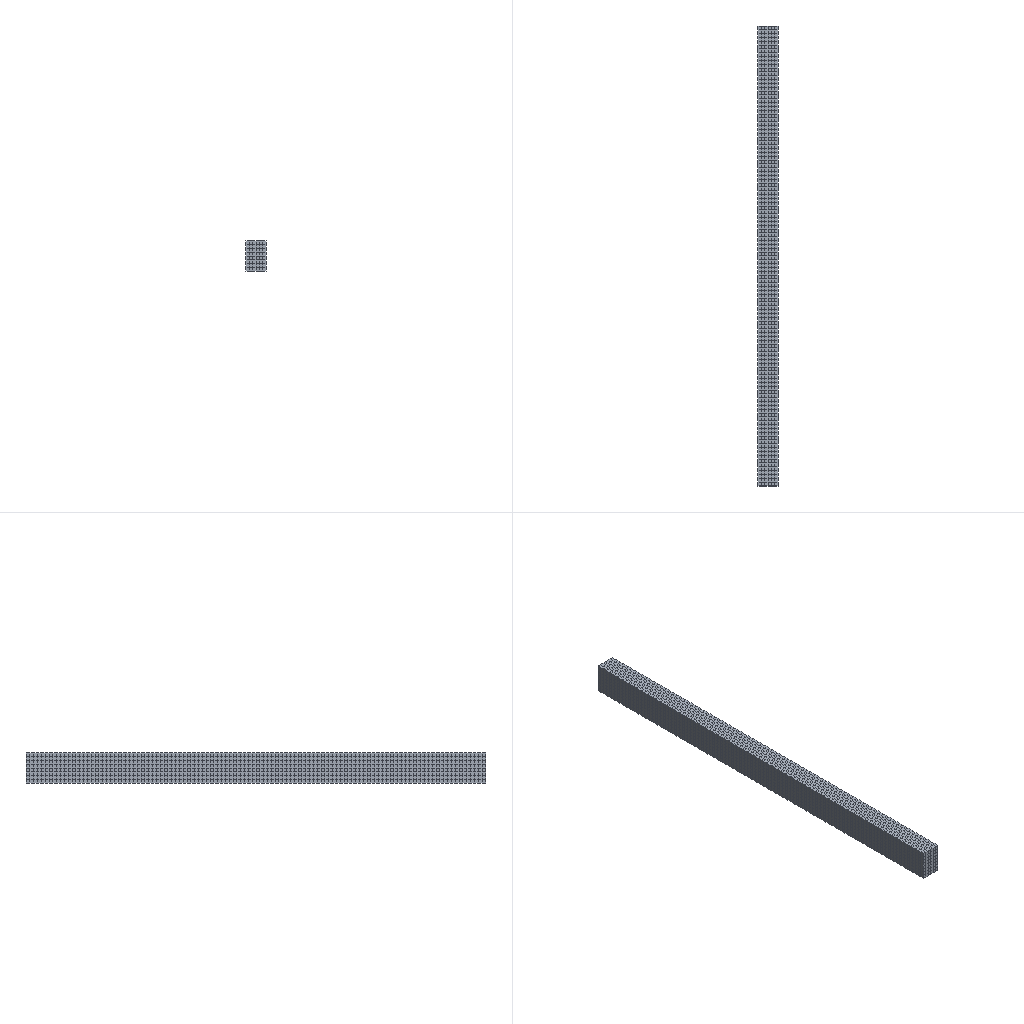Simulation study | ansys workbench
Ansys APDL input file, long lists of numbers shortened:
/batch
/config,noeldb,1     ! force off writing results to database
*get,_wallstrt,active,,time,wall
! ANSYS input file written by Workbench version 2022 R1
! File used for geometry attach: F:\ansys（分析文件汇总)\简支梁有限元分析\零件3.STEP
/title,111--____ (C5)
! ****** Begin Custom Load Command Snippet ******
/COM, ACT Extensions:
/COM,     LSDYNA, 2021.1
/COM,
! ****** End   Custom Load Command Snippet ******
*DIM,_wb_ProjectScratch_dir,string,248
_wb_ProjectScratch_dir(1) = 'F:\ansys（分析文件汇总)\简支梁有限元分析\_ProjectScratch\ScrC7EA\'
*DIM,_wb_SolverFiles_dir,string,248
_wb_SolverFiles_dir(1) = 'F:\ansys（分析文件汇总)\简支梁有限元分析\111_files\dp0\SYS-1\MECH\'
*DIM,_wb_userfiles_dir,string,248
_wb_userfiles_dir(1) = 'F:\ansys（分析文件汇总)\简支梁有限元分析\111_files\user_files\'
/com,--- Data in consistent NMM units. See Solving Units in the help system for more information.
/units,MPA
/nopr
/wb,file,start              !  signify a WB generated input file
/prep7
! Turn off shape checking because checks already performed inside WB mesher.
! See help system for more information.
SHPP,OFF,,NOWARN
/nolist
etcon,set             ! allow ANSYS to choose best KEYOP's for 180x elements, resets any applicable keyopt to MAPDL defaults
/com,*********** Nodes for the whole assembly ***********
nblock,3,,127902
(1i9,3e20.9e3)
        1    -5.133333333E+01     1.215000000E+03     8.485714286E+01
! (116274 more lines like these left out)
-1
/wb,elem,start            !  set before creation of elements
/com,*********** Elements for Body 1 "__3-FreeParts|__1[2]" ***********
et,1,186
keyo,1,2,1          ! set full integration on SOLID186
eblock,19,solid,,10080
(19i9)
        1        1        1        1        0        0        0        0       20        0    15121    69851    80547    80568    81290    79093    80560    80569    82000
! (20159 more lines like these left out)
-1
/com,*********** Elements for Body 2 "__3-FreeParts|__1[1]" ***********
et,2,186
keyo,2,2,1          ! set full integration on SOLID186
eblock,19,solid,,5040
(19i9)
        2        2        2        2        0        0        0        0       20        0        1        1     5405     5441     5449     4563     5418     5440     5799
! (10079 more lines like these left out)
-1
/com,*********** Elements for Body 3 "__3-FreeParts|__1[3]" ***********
et,3,186
keyo,3,2,1          ! set full integration on SOLID186
eblock,19,solid,,10080
(19i9)
        3        3        3        3        0        0        0        0       20        0     5041    23426    35471    34596    34515    32668    35563    34595    34594
! (20159 more lines like these left out)
-1
/wb,elem,end               !  done creating elements
/com,*********** Send User Defined Coordinate System(s) ***********
csys,0
toffst,273.15,  ! Temperature offset from absolute zero
/com,*********** Set Reference Temperature ***********
tref,22.
/wb,mat,start              !  starting to send materials
/com,*********** Send Materials ***********
Temperature = 'TEMP' ! Temperature
MP,DENS,1,7.85e-09,	! tonne mm^-3
MP,ALPX,1,1.2e-05,	! C^-1
MP,C,1,434000000,	! mm^2 s^-2 C^-1
MP,KXX,1,60.5,	! tonne mm s^-3 C^-1
MP,RSVX,1,0.00017,	! ohm mm
MP,EX,1,200000,	! tonne s^-2 mm^-1
MP,NUXY,1,0.3,
MP,MURX,1,10000,
Temperature = 'TEMP' ! Temperature
MP,DENS,2,7.85e-09,	! tonne mm^-3
MP,ALPX,2,1.2e-05,	! C^-1
MP,C,2,434000000,	! mm^2 s^-2 C^-1
MP,KXX,2,60.5,	! tonne mm s^-3 C^-1
MP,RSVX,2,0.00017,	! ohm mm
MP,EX,2,200000,	! tonne s^-2 mm^-1
MP,NUXY,2,0.3,
MP,MURX,2,10000,
Temperature = 'TEMP' ! Temperature
MP,DENS,3,7.85e-09,	! tonne mm^-3
MP,ALPX,3,1.2e-05,	! C^-1
MP,C,3,434000000,	! mm^2 s^-2 C^-1
MP,KXX,3,60.5,	! tonne mm s^-3 C^-1
MP,RSVX,3,0.00017,	! ohm mm
MP,EX,3,200000,	! tonne s^-2 mm^-1
MP,NUXY,3,0.3,
MP,MURX,3,10000,
/wb,mat,end                !  done sending materials
!************************* Model Summary ********************
!__3-FreeParts|__1[2],	结构钢,	matid,	1
!__3-FreeParts|__1[1],	结构钢,	matid,	2
!__3-FreeParts|__1[3],	结构钢,	matid,	3
!************************* End Model Summary ********************
! get the diagonal of the bounding box. Needed later for other things
*get,_xmin,node,,mnloc,x
*get,_ymin,node,,mnloc,y
*get,_zmin,node,,mnloc,z
*get,_xmax,node,,mxloc,x
*get,_ymax,node,,mxloc,y
*get,_zmax,node,,mxloc,z
_ASMDIAG=(_xmax-_xmin)*(_xmax-_xmin)+(_ymax-_ymin)*(_ymax-_ymin)+(_zmax-_zmin)*(_zmax-_zmin)
_ASMDIAG=SQRT(_ASMDIAG)
/wb,contact,start          !  starting to send contact
/com,*********** Create Contact "接触区域" ***********
/com,            Real Constant Set For Above Contact Is 5 & 4
*set,tid,5
*set,cid,4
r,tid
r,cid
et,tid,170
et,cid,174
eblock,10,,,126
(15i9)
    35157        5        5        5        0    80295    80309    80434    80294   113054   113082   113052   113051
! (125 more lines like these left out)
-1
eblock,10,,,126
(15i9)
    35283        4        4        4        0    80295    80309    80434    80294   113054   113082   113052   113051
! (125 more lines like these left out)
-1
eblock,10,,,126
(15i9)
    35409        4        5        4        0     5448     5314     5150     5149    21856    21535    21532    21533
! (125 more lines like these left out)
-1
eblock,10,,,126
(15i9)
    35535        5        4        5        0     5448     5314     5150     5149    21856    21535    21532    21533
! (125 more lines like these left out)
-1
keyo,cid,8,2               ! auto create asymmetric contact (from Program Controlled setting)
keyo,cid,10,0              ! adjust contact stiffness each NR iteration (from Program Controlled setting)
keyo,cid,12,5              ! bonded always
keyo,cid,18,1              ! small sliding turned on by application
keyo,cid,2,0               ! augmented Lagrange (from Program Controlled setting)
keyo,cid,4,0               ! on Gauss point (from Program Controlled setting)
keyo,cid,9,1               ! ignore initial gaps/penetration
keyo,cid,7,0               ! No Prediction
rmod,tid,3,10.      ! FKN
rmod,tid,5,0.       ! ICONT
rmod,tid,6,0.       ! PINB
rmod,tid,10,0.      ! CNOF
rmod,tid,12,0.      ! FKT
rmod,tid,36,72      ! WB DSID
rmod,cid,3,10.      ! FKN
rmod,cid,5,0.       ! ICONT
rmod,cid,6,0.       ! PINB
rmod,cid,10,0.      ! CNOF
rmod,cid,12,0.      ! FKT
rmod,cid,36,72      ! WB DSID
/com,*********** Create Contact "接触区域 2" ***********
/com,            Real Constant Set For Above Contact Is 7 & 6
*set,tid,7
*set,cid,6
r,tid
r,cid
et,tid,170
et,cid,174
eblock,10,,,126
(15i9)
    35661        7        7        7        0     5295     5179     5303     5304    21592    21593    21834    21819
! (125 more lines like these left out)
-1
eblock,10,,,126
(15i9)
    35787        6        6        6        0     5295     5179     5303     5304    21592    21593    21834    21819
! (125 more lines like these left out)
-1
eblock,10,,,126
(15i9)
    35913        6        7        6        0    35457    35459    35575    35458    69637    69641    69638    69636
! (125 more lines like these left out)
-1
eblock,10,,,126
(15i9)
    36039        7        6        7        0    35457    35459    35575    35458    69637    69641    69638    69636
! (125 more lines like these left out)
-1
keyo,cid,8,2               ! auto create asymmetric contact (from Program Controlled setting)
keyo,cid,10,0              ! adjust contact stiffness each NR iteration (from Program Controlled setting)
keyo,cid,12,5              ! bonded always
keyo,cid,18,1              ! small sliding turned on by application
keyo,cid,2,0               ! augmented Lagrange (from Program Controlled setting)
keyo,cid,4,0               ! on Gauss point (from Program Controlled setting)
keyo,cid,9,1               ! ignore initial gaps/penetration
keyo,cid,7,0               ! No Prediction
rmod,tid,3,10.      ! FKN
rmod,tid,5,0.       ! ICONT
rmod,tid,6,0.       ! PINB
rmod,tid,10,0.      ! CNOF
rmod,tid,12,0.      ! FKT
rmod,tid,36,75      ! WB DSID
rmod,cid,3,10.      ! FKN
rmod,cid,5,0.       ! ICONT
rmod,cid,6,0.       ! PINB
rmod,cid,10,0.      ! CNOF
rmod,cid,12,0.      ! FKT
rmod,cid,36,75      ! WB DSID
nsel,all
esel,all
/wb,contact,end            !  done creating contacts
/golist
/wb,load,start             !  starting to send loads
/com,*********** Fixed Supports ***********
CMBLOCK,_FIXEDSU,NODE,       19
(8i10)
     80293     80561     80562     80563     80564     80565     80566     80567
     80568     80569    113050    113574    113576    113578    113580    113582
    113584    113586    113588
cmsel,s,_FIXEDSU
d,all,all
nsel,all
/com,******* Constant Zero Displacement X *******
CMBLOCK,_DISPZEROUX,NODE,       19
(8i10)
     33883     34604     34605     34606     34607     34608     34609     34610
     34611     34612     66654     68024     68026     68028     68030     68032
     68034     68036     68038
cmsel,s,_DISPZEROUX
d,all,ux,0
nsel,all
/com,******* Constant Zero Displacement Z *******
CMBLOCK,_DISPZEROUZ,NODE,       19
(8i10)
     33883     34604     34605     34606     34607     34608     34609     34610
     34611     34612     66654     68024     68026     68028     68030     68032
     68034     68036     68038
cmsel,s,_DISPZEROUZ
d,all,uz,0
nsel,all
/com,*********** Define Force Using Surface Effect Elements ***********
local,12,0,0.,0.,0.,0.,0.,0.
csys,0
et,8,154
eblock,10,,,360
(15i9)
    36165        8        8        8       12     5441     5449     5799     5440    22104    22120    22102    22101
! (359 more lines like these left out)
-1
esel,s,type,,8
keyop,8,2,1                ! Apply load in local coordinate system
keyop,8,7,1                ! Use original area so load is constant in large deformation
esel,all
/gst,on,on
fini
*get,_numnode,node,0,count
*get,_numelem,elem,0,count
*get, _MAXELEMNUM, elem, 0, NUM, MAX
*get, _MAXNODENUM, node, 0, NUM, MAX
*get, _MAXELEMTYPE, etyp, 0, NUM, MAX
*get, _MAXREALCONST, real, 0, NUM, MAX
/go
/wb,load,end               !  done creating loads
/com,--- Number of total nodes = %_numnode%
/com,--- Number of contact elements = 1368
/com,--- Number of spring elements = 0
/com,--- Number of bearing elements = 0
/com,--- Number of solid elements = 25200
/com,--- Number of condensed parts = 0
/com,--- Number of total elements = %_numelem%
*get,_wallbsol,active,,time,wall
/com,****************************************************************************
/com,*************************    SOLUTION       ********************************
/com,****************************************************************************
/solu
antype,0                   ! static analysis
_thickRatio=  1     ! Ratio of thick parts in the model
eqsl,pcg,1e-8,,,,,,1
cntr,print,1               ! print out contact info and also make no initial contact an error
dmpoption,emat,no             ! Don't combine emat file for DANSYS
dmpoption,esav,no             ! Don't combine esav file for DANSYS
nldiag,cont,iter           ! print out contact info each equilibrium iteration
rescontrol,,none                 ! Do not keep any restart files
/com,****************************************************
/com,******************* SOLVE FOR LS 1 OF 1 ****************
esel,s,type,,8
nsle
sfe,all,1,pres,1,-4.38061479654879e-017
sfe,all,2,pres,1,0.
sfe,all,3,pres,1,-0.4167
nsel,all
esel,all
/nopr
/gopr
nsub,1,1,1
time,1.
outres,erase
outres,all,none
outres,nsol,all,
outres,rsol,all
outres,eangl,all
outres,etmp,all
outres,veng,all
outres,strs,all,
outres,epel,all,
outres,eppl,all,
outres,cont,all,
! *********** WB SOLVE COMMAND ***********
! check interactive state
*get,ANSINTER_,active,,int
*if,ANSINTER_,ne,0,then
/eof
*endif
solve
/com *************** Write FE CONNECTORS *********
CEWRITE,file,ce,,INTE
/com,****************************************************
/com,*************** FINISHED SOLVE FOR LS 1 *************
*get,_wallasol,active,,time,wall
/nopr
*get,_numnode,node,0,count
*get,_numelem,elem,0,count
*get, _MAXELEMNUM, elem, 0, NUM, MAX
*get, _MAXNODENUM, node, 0, NUM, MAX,,,INTERNAL
*get, _MAXELEMTYPE, etyp, 0, NUM, MAX
*get, _MAXREALCONST, real, 0, NUM, MAX
/gopr
*get,_PCGITER,active,,solu,cgiter
/post1
xmlo,ENCODING,ISO-8859-1
xmlo,parm
/xml,parm,xml
fini
/gopr
*get,_walldone,active,,time,wall
_preptime=(_wallbsol-_wallstrt)*3600
_solvtime=(_wallasol-_wallbsol)*3600
_posttime=(_walldone-_wallasol)*3600
_totaltim=(_walldone-_wallstrt)*3600
*get,_dlbratio,active,0,solu,dlbr
*get,_combtime,active,0,solu,comb
*get,_ssmode,active,0,solu,ssmm
*get,_ndofs,active,0,solu,ndof
*get,_sol_end_time,active,0,set,time
*if,_sol_end_time,eq,1.,then
/fclean				!clean distributed files
*endif
/com,--- Total number of nodes = %_numnode%
/com,--- Total number of elements = %_numelem%
/com,--- Element load balance ratio = %_dlbratio%
/com,--- Time to combine distributed files = %_combtime%
/com,--- Sparse memory mode = %_ssmode%
/com,--- Number of DOF = %_ndofs%
/wb,file,end               ! done with WB generated input